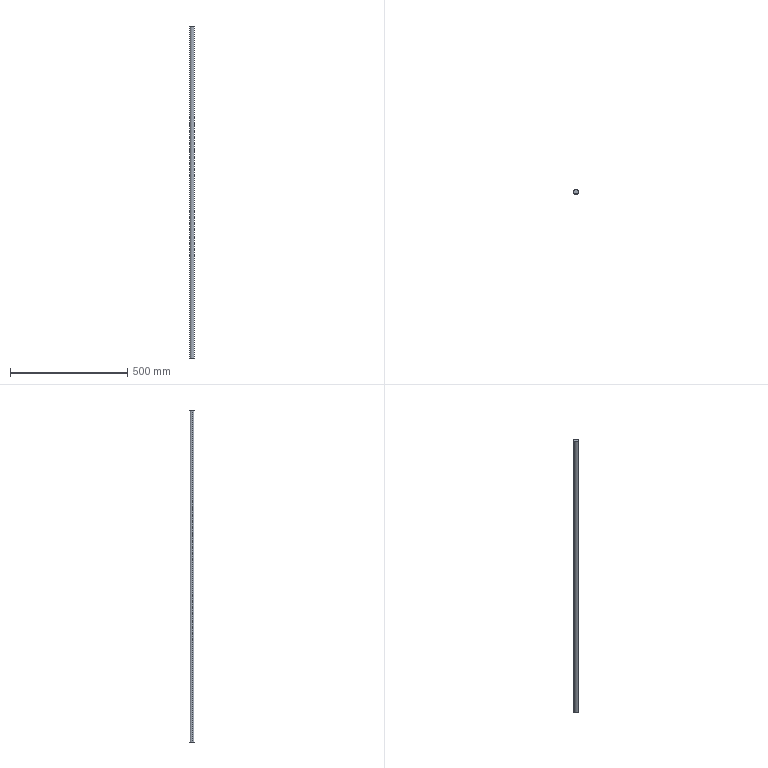Part | SolidWorks | features BaseBody 1, ICE 1 | 1 solid | 4 faces | box 20 x 20 x 1414 mm | volume 444221 mm3 | cylinder 2 | plane 2 | commonest cylinder face diameters 20 x2
STEP:
#1=CARTESIAN_POINT('',(10.,0.,497.));
#2=VERTEX_POINT('',#1);
#3=CARTESIAN_POINT('',(-10.,0.,497.));
#4=VERTEX_POINT('',#3);
#5=CARTESIAN_POINT('',(0.,0.,497.));
#6=DIRECTION('',(0.,0.,1.));
#7=DIRECTION('',(1.,0.,0.));
#8=AXIS2_PLACEMENT_3D('',#5,#6,#7);
#9=CIRCLE('',#8,10.);
#10=EDGE_CURVE('',#2,#4,#9,.T.);
#11=ORIENTED_EDGE('',*,*,#10,.F.);
#12=CARTESIAN_POINT('',(10.,0.,-917.));
#13=VERTEX_POINT('',#12);
#14=CARTESIAN_POINT('',(10.,0.,892.));
#15=DIRECTION('',(0.,0.,-1.));
#16=VECTOR('',#15,1000.);
#17=LINE('',#14,#16);
#18=EDGE_CURVE('',#2,#13,#17,.T.);
#19=ORIENTED_EDGE('',*,*,#18,.T.);
#20=CARTESIAN_POINT('',(-10.,0.,-917.));
#21=VERTEX_POINT('',#20);
#22=CARTESIAN_POINT('',(0.,0.,-917.));
#23=DIRECTION('',(0.,0.,1.));
#24=DIRECTION('',(-1.,0.,0.));
#25=AXIS2_PLACEMENT_3D('',#22,#23,#24);
#26=CIRCLE('',#25,10.);
#27=EDGE_CURVE('',#13,#21,#26,.T.);
#28=ORIENTED_EDGE('',*,*,#27,.T.);
#29=CARTESIAN_POINT('',(-10.,0.,892.));
#30=DIRECTION('',(0.,0.,-1.));
#31=VECTOR('',#30,1000.);
#32=LINE('',#29,#31);
#33=EDGE_CURVE('',#4,#21,#32,.T.);
#34=ORIENTED_EDGE('',*,*,#33,.F.);
#35=EDGE_LOOP('',(#11,#19,#28,#34));
#36=FACE_OUTER_BOUND('',#35,.T.);
#37=CARTESIAN_POINT('',(0.,0.,892.));
#38=DIRECTION('',(0.,0.,-1.));
#39=DIRECTION('',(-1.,0.,0.));
#40=AXIS2_PLACEMENT_3D('',#37,#38,#39);
#41=CYLINDRICAL_SURFACE('',#40,10.);
#42=ADVANCED_FACE('',(#36),#41,.T.);
#43=ORIENTED_EDGE('',*,*,#18,.F.);
#44=CARTESIAN_POINT('',(0.,0.,497.));
#45=DIRECTION('',(0.,0.,1.));
#46=DIRECTION('',(1.,0.,0.));
#47=AXIS2_PLACEMENT_3D('',#44,#45,#46);
#48=CIRCLE('',#47,10.);
#49=EDGE_CURVE('',#4,#2,#48,.T.);
#50=ORIENTED_EDGE('',*,*,#49,.F.);
#51=ORIENTED_EDGE('',*,*,#33,.T.);
#52=CARTESIAN_POINT('',(0.,0.,-917.));
#53=DIRECTION('',(0.,0.,1.));
#54=DIRECTION('',(-1.,0.,0.));
#55=AXIS2_PLACEMENT_3D('',#52,#53,#54);
#56=CIRCLE('',#55,10.);
#57=EDGE_CURVE('',#21,#13,#56,.T.);
#58=ORIENTED_EDGE('',*,*,#57,.T.);
#59=EDGE_LOOP('',(#43,#50,#51,#58));
#60=FACE_OUTER_BOUND('',#59,.T.);
#61=CARTESIAN_POINT('',(0.,0.,892.));
#62=DIRECTION('',(0.,0.,-1.));
#63=DIRECTION('',(-1.,0.,0.));
#64=AXIS2_PLACEMENT_3D('',#61,#62,#63);
#65=CYLINDRICAL_SURFACE('',#64,10.);
#66=ADVANCED_FACE('',(#60),#65,.T.);
#67=ORIENTED_EDGE('',*,*,#57,.F.);
#68=ORIENTED_EDGE('',*,*,#27,.F.);
#69=EDGE_LOOP('',(#67,#68));
#70=FACE_OUTER_BOUND('',#69,.T.);
#71=CARTESIAN_POINT('',(0.,0.,-917.));
#72=DIRECTION('',(0.,0.,-1.));
#73=DIRECTION('',(-1.,0.,0.));
#74=AXIS2_PLACEMENT_3D('',#71,#72,#73);
#75=PLANE('',#74);
#76=ADVANCED_FACE('',(#70),#75,.T.);
#77=ORIENTED_EDGE('',*,*,#49,.T.);
#78=ORIENTED_EDGE('',*,*,#10,.T.);
#79=EDGE_LOOP('',(#77,#78));
#80=FACE_OUTER_BOUND('',#79,.T.);
#81=CARTESIAN_POINT('',(0.,0.,497.));
#82=DIRECTION('',(0.,0.,1.));
#83=DIRECTION('',(1.,0.,0.));
#84=AXIS2_PLACEMENT_3D('',#81,#82,#83);
#85=PLANE('',#84);
#86=ADVANCED_FACE('',(#80),#85,.T.);
#87=CLOSED_SHELL('',(#42,#66,#76,#86));
#88=MANIFOLD_SOLID_BREP('',#87);
#89=CARTESIAN_POINT('',(0.,0.,0.));
#90=DIRECTION('',(0.,0.,1.));
#91=DIRECTION('',(1.,0.,0.));
#92=AXIS2_PLACEMENT_3D('',#89,#90,#91);
#93=(LENGTH_UNIT()NAMED_UNIT(*)SI_UNIT(.MILLI.,.METRE.));
#94=UNCERTAINTY_MEASURE_WITH_UNIT(LENGTH_MEASURE(0.00001),#93,'','');
#95=(NAMED_UNIT(*)PLANE_ANGLE_UNIT()SI_UNIT($,.RADIAN.));
#96=(NAMED_UNIT(*)SI_UNIT($,.STERADIAN.)SOLID_ANGLE_UNIT());
#97=(GEOMETRIC_REPRESENTATION_CONTEXT(3)GLOBAL_UNCERTAINTY_ASSIGNED_CONTEXT((#94))GLOBAL_UNIT_ASSIGNED_CONTEXT((#93,#95,#96))REPRESENTATION_CONTEXT('',''));
#98=ADVANCED_BREP_SHAPE_REPRESENTATION('',(#88,#92),#97);